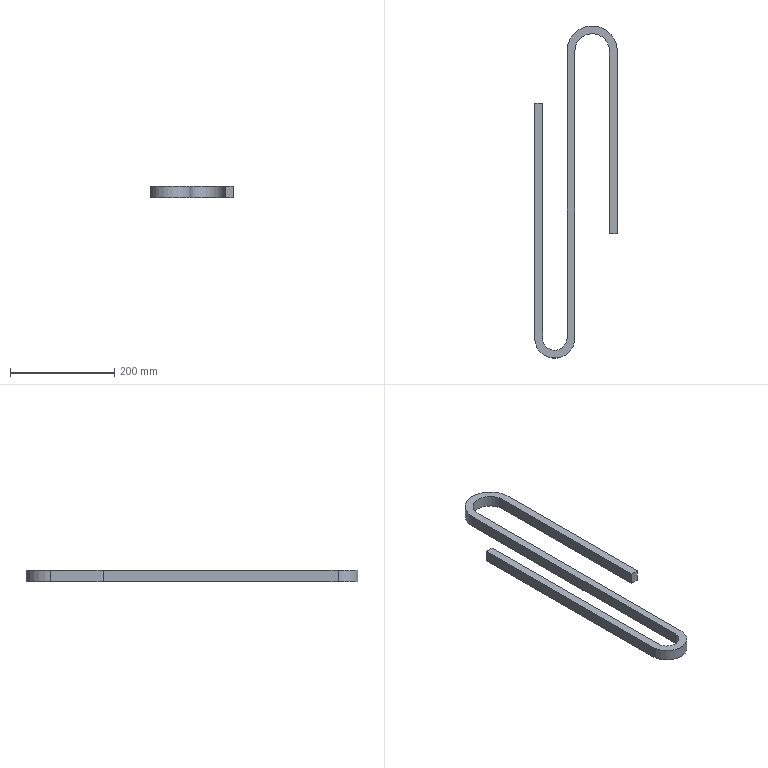Part | STEP file | PN_0043 (chain bar) | 1 solid | 14 faces | box 158.46 x 636.775 x 22 mm | volume 522937 mm3 | plane 10 | cylinder 4 | commonest cylinder face diameters 46.91 x1 66.28 x1 77.09 x1 96.46 x1
STEP:
#1=CARTESIAN_POINT('',(0.,0.,0.));
#2=DIRECTION('',(0.,0.,1.));
#3=DIRECTION('',(1.,0.,0.));
#4=AXIS2_PLACEMENT_3D('',#1,#2,#3);
#5=CARTESIAN_POINT('',(-95.14,150.,11.));
#6=VERTEX_POINT('',#5);
#7=CARTESIAN_POINT('',(-95.14,150.,-11.));
#8=VERTEX_POINT('',#7);
#9=CARTESIAN_POINT('',(-95.14,150.,-11.));
#10=DIRECTION('',(0.,0.,-1.));
#11=VECTOR('',#10,1.);
#12=LINE('',#9,#11);
#13=CARTESIAN_POINT('',(-95.14,150.,-11.));
#14=DIRECTION('',(1.,0.,0.));
#15=DIRECTION('',(0.,1.,0.));
#16=AXIS2_PLACEMENT_3D('',#13,#14,#15);
#17=PLANE('',#16);
#18=CARTESIAN_POINT('',(0.,0.));
#19=DIRECTION('',(0.,-1.));
#20=VECTOR('',#19,1.);
#21=LINE('',#18,#20);
#22=(GEOMETRIC_REPRESENTATION_CONTEXT(2)PARAMETRIC_REPRESENTATION_CONTEXT()REPRESENTATION_CONTEXT('',''));
#23=DEFINITIONAL_REPRESENTATION('',(#21),#22);
#24=PCURVE('',#17,#23);
#25=CARTESIAN_POINT('',(-71.685,150.,0.));
#26=DIRECTION('',(0.,0.,-1.));
#27=DIRECTION('',(-1.,0.,0.));
#28=AXIS2_PLACEMENT_3D('',#25,#26,#27);
#29=CYLINDRICAL_SURFACE('',#28,23.455);
#30=CARTESIAN_POINT('',(6.283,11.));
#31=DIRECTION('',(0.,1.));
#32=VECTOR('',#31,1.);
#33=LINE('',#30,#32);
#34=(GEOMETRIC_REPRESENTATION_CONTEXT(2)PARAMETRIC_REPRESENTATION_CONTEXT()REPRESENTATION_CONTEXT('',''));
#35=DEFINITIONAL_REPRESENTATION('',(#33),#34);
#36=PCURVE('',#29,#35);
#37=SURFACE_CURVE('',#12,(#24,#36),.PCURVE_S1.);
#38=EDGE_CURVE('',#6,#8,#37,.T.);
#39=ORIENTED_EDGE('',*,*,#38,.T.);
#40=CARTESIAN_POINT('',(-95.14,600.,-11.));
#41=VERTEX_POINT('',#40);
#42=CARTESIAN_POINT('',(-95.14,150.,-11.));
#43=DIRECTION('',(0.,1.,0.));
#44=VECTOR('',#43,1.);
#45=LINE('',#42,#44);
#46=CARTESIAN_POINT('',(0.,0.));
#47=DIRECTION('',(1.,0.));
#48=VECTOR('',#47,1.);
#49=LINE('',#46,#48);
#50=(GEOMETRIC_REPRESENTATION_CONTEXT(2)PARAMETRIC_REPRESENTATION_CONTEXT()REPRESENTATION_CONTEXT('',''));
#51=DEFINITIONAL_REPRESENTATION('',(#49),#50);
#52=PCURVE('',#17,#51);
#53=CARTESIAN_POINT('',(48.23,700.,-11.));
#54=DIRECTION('',(0.,0.,1.));
#55=DIRECTION('',(1.,0.,0.));
#56=AXIS2_PLACEMENT_3D('',#53,#54,#55);
#57=PLANE('',#56);
#58=CARTESIAN_POINT('',(-143.37,-550.));
#59=DIRECTION('',(0.,1.));
#60=VECTOR('',#59,1.);
#61=LINE('',#58,#60);
#62=(GEOMETRIC_REPRESENTATION_CONTEXT(2)PARAMETRIC_REPRESENTATION_CONTEXT()REPRESENTATION_CONTEXT('',''));
#63=DEFINITIONAL_REPRESENTATION('',(#61),#62);
#64=PCURVE('',#57,#63);
#65=SURFACE_CURVE('',#45,(#52,#64),.PCURVE_S1.);
#66=EDGE_CURVE('',#8,#41,#65,.T.);
#67=ORIENTED_EDGE('',*,*,#66,.T.);
#68=CARTESIAN_POINT('',(-95.14,600.,11.));
#69=VERTEX_POINT('',#68);
#70=CARTESIAN_POINT('',(-95.14,600.,-11.));
#71=DIRECTION('',(0.,0.,-1.));
#72=VECTOR('',#71,1.);
#73=LINE('',#70,#72);
#74=CARTESIAN_POINT('',(450.,0.));
#75=DIRECTION('',(0.,-1.));
#76=VECTOR('',#75,1.);
#77=LINE('',#74,#76);
#78=(GEOMETRIC_REPRESENTATION_CONTEXT(2)PARAMETRIC_REPRESENTATION_CONTEXT()REPRESENTATION_CONTEXT('',''));
#79=DEFINITIONAL_REPRESENTATION('',(#77),#78);
#80=PCURVE('',#17,#79);
#81=CARTESIAN_POINT('',(-143.37,600.,0.));
#82=DIRECTION('',(0.,-1.,0.));
#83=DIRECTION('',(0.,0.,-1.));
#84=AXIS2_PLACEMENT_3D('',#81,#82,#83);
#85=PLANE('',#84);
#86=CARTESIAN_POINT('',(11.,48.23));
#87=DIRECTION('',(1.,0.));
#88=VECTOR('',#87,1.);
#89=LINE('',#86,#88);
#90=(GEOMETRIC_REPRESENTATION_CONTEXT(2)PARAMETRIC_REPRESENTATION_CONTEXT()REPRESENTATION_CONTEXT('',''));
#91=DEFINITIONAL_REPRESENTATION('',(#89),#90);
#92=PCURVE('',#85,#91);
#93=SURFACE_CURVE('',#73,(#80,#92),.PCURVE_S1.);
#94=EDGE_CURVE('',#69,#41,#93,.T.);
#95=ORIENTED_EDGE('',*,*,#94,.F.);
#96=CARTESIAN_POINT('',(-95.14,150.,11.));
#97=DIRECTION('',(0.,1.,0.));
#98=VECTOR('',#97,1.);
#99=LINE('',#96,#98);
#100=CARTESIAN_POINT('',(0.,22.));
#101=DIRECTION('',(1.,0.));
#102=VECTOR('',#101,1.);
#103=LINE('',#100,#102);
#104=(GEOMETRIC_REPRESENTATION_CONTEXT(2)PARAMETRIC_REPRESENTATION_CONTEXT()REPRESENTATION_CONTEXT('',''));
#105=DEFINITIONAL_REPRESENTATION('',(#103),#104);
#106=PCURVE('',#17,#105);
#107=CARTESIAN_POINT('',(48.23,700.,11.));
#108=DIRECTION('',(0.,0.,-1.));
#109=DIRECTION('',(-1.,0.,0.));
#110=AXIS2_PLACEMENT_3D('',#107,#108,#109);
#111=PLANE('',#110);
#112=CARTESIAN_POINT('',(143.37,-550.));
#113=DIRECTION('',(0.,1.));
#114=VECTOR('',#113,1.);
#115=LINE('',#112,#114);
#116=(GEOMETRIC_REPRESENTATION_CONTEXT(2)PARAMETRIC_REPRESENTATION_CONTEXT()REPRESENTATION_CONTEXT('',''));
#117=DEFINITIONAL_REPRESENTATION('',(#115),#116);
#118=PCURVE('',#111,#117);
#119=SURFACE_CURVE('',#99,(#106,#118),.PCURVE_S1.);
#120=EDGE_CURVE('',#6,#69,#119,.T.);
#121=ORIENTED_EDGE('',*,*,#120,.F.);
#122=EDGE_LOOP('',(#39,#67,#95,#121));
#123=FACE_BOUND('',#122,.T.);
#124=ADVANCED_FACE('',(#123),#17,.T.);
#125=CARTESIAN_POINT('',(-110.23,150.,-11.));
#126=VERTEX_POINT('',#125);
#127=CARTESIAN_POINT('',(-110.23,150.,11.));
#128=VERTEX_POINT('',#127);
#129=CARTESIAN_POINT('',(-110.23,150.,-11.));
#130=DIRECTION('',(0.,0.,1.));
#131=VECTOR('',#130,1.);
#132=LINE('',#129,#131);
#133=CARTESIAN_POINT('',(-110.23,150.,-11.));
#134=DIRECTION('',(-1.,0.,0.));
#135=DIRECTION('',(0.,-1.,0.));
#136=AXIS2_PLACEMENT_3D('',#133,#134,#135);
#137=PLANE('',#136);
#138=CARTESIAN_POINT('',(0.,0.));
#139=DIRECTION('',(0.,1.));
#140=VECTOR('',#139,1.);
#141=LINE('',#138,#140);
#142=(GEOMETRIC_REPRESENTATION_CONTEXT(2)PARAMETRIC_REPRESENTATION_CONTEXT()REPRESENTATION_CONTEXT('',''));
#143=DEFINITIONAL_REPRESENTATION('',(#141),#142);
#144=PCURVE('',#137,#143);
#145=CARTESIAN_POINT('',(-71.685,150.,0.));
#146=DIRECTION('',(0.,0.,-1.));
#147=DIRECTION('',(-1.,0.,0.));
#148=AXIS2_PLACEMENT_3D('',#145,#146,#147);
#149=CYLINDRICAL_SURFACE('',#148,38.545);
#150=CARTESIAN_POINT('',(6.283,11.));
#151=DIRECTION('',(0.,-1.));
#152=VECTOR('',#151,1.);
#153=LINE('',#150,#152);
#154=(GEOMETRIC_REPRESENTATION_CONTEXT(2)PARAMETRIC_REPRESENTATION_CONTEXT()REPRESENTATION_CONTEXT('',''));
#155=DEFINITIONAL_REPRESENTATION('',(#153),#154);
#156=PCURVE('',#149,#155);
#157=SURFACE_CURVE('',#132,(#144,#156),.PCURVE_S1.);
#158=EDGE_CURVE('',#126,#128,#157,.T.);
#159=ORIENTED_EDGE('',*,*,#158,.T.);
#160=CARTESIAN_POINT('',(-110.23,600.,11.));
#161=VERTEX_POINT('',#160);
#162=CARTESIAN_POINT('',(-110.23,150.,11.));
#163=DIRECTION('',(0.,1.,0.));
#164=VECTOR('',#163,1.);
#165=LINE('',#162,#164);
#166=CARTESIAN_POINT('',(0.,22.));
#167=DIRECTION('',(-1.,0.));
#168=VECTOR('',#167,1.);
#169=LINE('',#166,#168);
#170=(GEOMETRIC_REPRESENTATION_CONTEXT(2)PARAMETRIC_REPRESENTATION_CONTEXT()REPRESENTATION_CONTEXT('',''));
#171=DEFINITIONAL_REPRESENTATION('',(#169),#170);
#172=PCURVE('',#137,#171);
#173=CARTESIAN_POINT('',(158.46,-550.));
#174=DIRECTION('',(0.,1.));
#175=VECTOR('',#174,1.);
#176=LINE('',#173,#175);
#177=(GEOMETRIC_REPRESENTATION_CONTEXT(2)PARAMETRIC_REPRESENTATION_CONTEXT()REPRESENTATION_CONTEXT('',''));
#178=DEFINITIONAL_REPRESENTATION('',(#176),#177);
#179=PCURVE('',#111,#178);
#180=SURFACE_CURVE('',#165,(#172,#179),.PCURVE_S1.);
#181=EDGE_CURVE('',#128,#161,#180,.T.);
#182=ORIENTED_EDGE('',*,*,#181,.T.);
#183=CARTESIAN_POINT('',(-110.23,600.,-11.));
#184=VERTEX_POINT('',#183);
#185=CARTESIAN_POINT('',(-110.23,600.,-11.));
#186=DIRECTION('',(0.,0.,1.));
#187=VECTOR('',#186,1.);
#188=LINE('',#185,#187);
#189=CARTESIAN_POINT('',(-450.,0.));
#190=DIRECTION('',(0.,1.));
#191=VECTOR('',#190,1.);
#192=LINE('',#189,#191);
#193=(GEOMETRIC_REPRESENTATION_CONTEXT(2)PARAMETRIC_REPRESENTATION_CONTEXT()REPRESENTATION_CONTEXT('',''));
#194=DEFINITIONAL_REPRESENTATION('',(#192),#193);
#195=PCURVE('',#137,#194);
#196=CARTESIAN_POINT('',(11.,33.14));
#197=DIRECTION('',(-1.,0.));
#198=VECTOR('',#197,1.);
#199=LINE('',#196,#198);
#200=(GEOMETRIC_REPRESENTATION_CONTEXT(2)PARAMETRIC_REPRESENTATION_CONTEXT()REPRESENTATION_CONTEXT('',''));
#201=DEFINITIONAL_REPRESENTATION('',(#199),#200);
#202=PCURVE('',#85,#201);
#203=SURFACE_CURVE('',#188,(#195,#202),.PCURVE_S1.);
#204=EDGE_CURVE('',#184,#161,#203,.T.);
#205=ORIENTED_EDGE('',*,*,#204,.F.);
#206=CARTESIAN_POINT('',(-110.23,150.,-11.));
#207=DIRECTION('',(0.,1.,0.));
#208=VECTOR('',#207,1.);
#209=LINE('',#206,#208);
#210=CARTESIAN_POINT('',(0.,0.));
#211=DIRECTION('',(-1.,0.));
#212=VECTOR('',#211,1.);
#213=LINE('',#210,#212);
#214=(GEOMETRIC_REPRESENTATION_CONTEXT(2)PARAMETRIC_REPRESENTATION_CONTEXT()REPRESENTATION_CONTEXT('',''));
#215=DEFINITIONAL_REPRESENTATION('',(#213),#214);
#216=PCURVE('',#137,#215);
#217=CARTESIAN_POINT('',(-158.46,-550.));
#218=DIRECTION('',(0.,1.));
#219=VECTOR('',#218,1.);
#220=LINE('',#217,#219);
#221=(GEOMETRIC_REPRESENTATION_CONTEXT(2)PARAMETRIC_REPRESENTATION_CONTEXT()REPRESENTATION_CONTEXT('',''));
#222=DEFINITIONAL_REPRESENTATION('',(#220),#221);
#223=PCURVE('',#57,#222);
#224=SURFACE_CURVE('',#209,(#216,#223),.PCURVE_S1.);
#225=EDGE_CURVE('',#126,#184,#224,.T.);
#226=ORIENTED_EDGE('',*,*,#225,.F.);
#227=EDGE_LOOP('',(#159,#182,#205,#226));
#228=FACE_BOUND('',#227,.T.);
#229=ADVANCED_FACE('',(#228),#137,.T.);
#230=CARTESIAN_POINT('',(-48.23,150.,11.));
#231=VERTEX_POINT('',#230);
#232=CARTESIAN_POINT('',(-71.685,150.,11.));
#233=DIRECTION('',(0.,0.,-1.));
#234=DIRECTION('',(-1.,0.,0.));
#235=AXIS2_PLACEMENT_3D('',#232,#233,#234);
#236=CIRCLE('',#235,23.455);
#237=CARTESIAN_POINT('',(0.,-11.));
#238=DIRECTION('',(1.,0.));
#239=VECTOR('',#238,1.);
#240=LINE('',#237,#239);
#241=(GEOMETRIC_REPRESENTATION_CONTEXT(2)PARAMETRIC_REPRESENTATION_CONTEXT()REPRESENTATION_CONTEXT('',''));
#242=DEFINITIONAL_REPRESENTATION('',(#240),#241);
#243=PCURVE('',#29,#242);
#244=CARTESIAN_POINT('',(119.915,-550.));
#245=DIRECTION('',(1.,0.));
#246=AXIS2_PLACEMENT_2D('',#244,#245);
#247=CIRCLE('',#246,23.455);
#248=(GEOMETRIC_REPRESENTATION_CONTEXT(2)PARAMETRIC_REPRESENTATION_CONTEXT()REPRESENTATION_CONTEXT('',''));
#249=DEFINITIONAL_REPRESENTATION('',(#247),#248);
#250=PCURVE('',#111,#249);
#251=SURFACE_CURVE('',#236,(#243,#250),.PCURVE_S1.);
#252=EDGE_CURVE('',#231,#6,#251,.T.);
#253=ORIENTED_EDGE('',*,*,#252,.T.);
#254=ORIENTED_EDGE('',*,*,#38,.T.);
#255=CARTESIAN_POINT('',(-48.23,150.,-11.));
#256=VERTEX_POINT('',#255);
#257=CARTESIAN_POINT('',(-71.685,150.,-11.));
#258=DIRECTION('',(0.,0.,-1.));
#259=DIRECTION('',(-1.,0.,0.));
#260=AXIS2_PLACEMENT_3D('',#257,#258,#259);
#261=CIRCLE('',#260,23.455);
#262=CARTESIAN_POINT('',(0.,11.));
#263=DIRECTION('',(1.,0.));
#264=VECTOR('',#263,1.);
#265=LINE('',#262,#264);
#266=(GEOMETRIC_REPRESENTATION_CONTEXT(2)PARAMETRIC_REPRESENTATION_CONTEXT()REPRESENTATION_CONTEXT('',''));
#267=DEFINITIONAL_REPRESENTATION('',(#265),#266);
#268=PCURVE('',#29,#267);
#269=CARTESIAN_POINT('',(-143.37,-550.));
#270=CARTESIAN_POINT('',(-143.37,-509.375));
#271=CARTESIAN_POINT('',(-108.188,-529.687));
#272=CARTESIAN_POINT('',(-73.005,-550.));
#273=CARTESIAN_POINT('',(-108.188,-570.313));
#274=CARTESIAN_POINT('',(-143.37,-590.625));
#275=CARTESIAN_POINT('',(-143.37,-550.));
#276=(BOUNDED_CURVE()B_SPLINE_CURVE(2,(#269,#270,#271,#272,#273,#274,#275),.UNSPECIFIED.,.T.,.F.)B_SPLINE_CURVE_WITH_KNOTS((1,2,2,2,2,1),(-2.094,0.,2.094,4.189,6.283,8.378),.UNSPECIFIED.)CURVE()GEOMETRIC_REPRESENTATION_ITEM()RATIONAL_B_SPLINE_CURVE((1.,0.5,1.,0.5,1.,0.5,1.))REPRESENTATION_ITEM(''));
#277=(GEOMETRIC_REPRESENTATION_CONTEXT(2)PARAMETRIC_REPRESENTATION_CONTEXT()REPRESENTATION_CONTEXT('',''));
#278=DEFINITIONAL_REPRESENTATION('',(#276),#277);
#279=PCURVE('',#57,#278);
#280=SURFACE_CURVE('',#261,(#268,#279),.PCURVE_S1.);
#281=EDGE_CURVE('',#256,#8,#280,.T.);
#282=ORIENTED_EDGE('',*,*,#281,.F.);
#283=CARTESIAN_POINT('',(-48.23,150.,-11.));
#284=DIRECTION('',(0.,0.,-1.));
#285=VECTOR('',#284,1.);
#286=LINE('',#283,#285);
#287=CARTESIAN_POINT('',(3.142,11.));
#288=DIRECTION('',(0.,1.));
#289=VECTOR('',#288,1.);
#290=LINE('',#287,#289);
#291=(GEOMETRIC_REPRESENTATION_CONTEXT(2)PARAMETRIC_REPRESENTATION_CONTEXT()REPRESENTATION_CONTEXT('',''));
#292=DEFINITIONAL_REPRESENTATION('',(#290),#291);
#293=PCURVE('',#29,#292);
#294=CARTESIAN_POINT('',(-48.23,700.,-11.));
#295=DIRECTION('',(-1.,0.,0.));
#296=DIRECTION('',(0.,-1.,0.));
#297=AXIS2_PLACEMENT_3D('',#294,#295,#296);
#298=PLANE('',#297);
#299=CARTESIAN_POINT('',(550.,0.));
#300=DIRECTION('',(0.,-1.));
#301=VECTOR('',#300,1.);
#302=LINE('',#299,#301);
#303=(GEOMETRIC_REPRESENTATION_CONTEXT(2)PARAMETRIC_REPRESENTATION_CONTEXT()REPRESENTATION_CONTEXT('',''));
#304=DEFINITIONAL_REPRESENTATION('',(#302),#303);
#305=PCURVE('',#298,#304);
#306=SURFACE_CURVE('',#286,(#293,#305),.PCURVE_S1.);
#307=EDGE_CURVE('',#231,#256,#306,.T.);
#308=ORIENTED_EDGE('',*,*,#307,.F.);
#309=EDGE_LOOP('',(#253,#254,#282,#308));
#310=FACE_BOUND('',#309,.F.);
#311=ADVANCED_FACE('',(#310),#29,.F.);
#312=CARTESIAN_POINT('',(-33.14,150.,-11.));
#313=VERTEX_POINT('',#312);
#314=CARTESIAN_POINT('',(-33.14,150.,11.));
#315=VERTEX_POINT('',#314);
#316=CARTESIAN_POINT('',(-33.14,150.,-11.));
#317=DIRECTION('',(0.,0.,1.));
#318=VECTOR('',#317,1.);
#319=LINE('',#316,#318);
#320=CARTESIAN_POINT('',(3.142,11.));
#321=DIRECTION('',(0.,-1.));
#322=VECTOR('',#321,1.);
#323=LINE('',#320,#322);
#324=(GEOMETRIC_REPRESENTATION_CONTEXT(2)PARAMETRIC_REPRESENTATION_CONTEXT()REPRESENTATION_CONTEXT('',''));
#325=DEFINITIONAL_REPRESENTATION('',(#323),#324);
#326=PCURVE('',#149,#325);
#327=CARTESIAN_POINT('',(-33.14,700.,-11.));
#328=DIRECTION('',(1.,0.,0.));
#329=DIRECTION('',(0.,1.,0.));
#330=AXIS2_PLACEMENT_3D('',#327,#328,#329);
#331=PLANE('',#330);
#332=CARTESIAN_POINT('',(-550.,0.));
#333=DIRECTION('',(0.,1.));
#334=VECTOR('',#333,1.);
#335=LINE('',#332,#334);
#336=(GEOMETRIC_REPRESENTATION_CONTEXT(2)PARAMETRIC_REPRESENTATION_CONTEXT()REPRESENTATION_CONTEXT('',''));
#337=DEFINITIONAL_REPRESENTATION('',(#335),#336);
#338=PCURVE('',#331,#337);
#339=SURFACE_CURVE('',#319,(#326,#338),.PCURVE_S1.);
#340=EDGE_CURVE('',#313,#315,#339,.T.);
#341=ORIENTED_EDGE('',*,*,#340,.T.);
#342=CARTESIAN_POINT('',(-71.685,150.,11.));
#343=DIRECTION('',(0.,0.,-1.));
#344=DIRECTION('',(-1.,0.,0.));
#345=AXIS2_PLACEMENT_3D('',#342,#343,#344);
#346=CIRCLE('',#345,38.545);
#347=CARTESIAN_POINT('',(0.,-11.));
#348=DIRECTION('',(1.,0.));
#349=VECTOR('',#348,1.);
#350=LINE('',#347,#349);
#351=(GEOMETRIC_REPRESENTATION_CONTEXT(2)PARAMETRIC_REPRESENTATION_CONTEXT()REPRESENTATION_CONTEXT('',''));
#352=DEFINITIONAL_REPRESENTATION('',(#350),#351);
#353=PCURVE('',#149,#352);
#354=CARTESIAN_POINT('',(119.915,-550.));
#355=DIRECTION('',(1.,0.));
#356=AXIS2_PLACEMENT_2D('',#354,#355);
#357=CIRCLE('',#356,38.545);
#358=(GEOMETRIC_REPRESENTATION_CONTEXT(2)PARAMETRIC_REPRESENTATION_CONTEXT()REPRESENTATION_CONTEXT('',''));
#359=DEFINITIONAL_REPRESENTATION('',(#357),#358);
#360=PCURVE('',#111,#359);
#361=SURFACE_CURVE('',#346,(#353,#360),.PCURVE_S1.);
#362=EDGE_CURVE('',#315,#128,#361,.T.);
#363=ORIENTED_EDGE('',*,*,#362,.T.);
#364=ORIENTED_EDGE('',*,*,#158,.F.);
#365=CARTESIAN_POINT('',(-71.685,150.,-11.));
#366=DIRECTION('',(0.,0.,-1.));
#367=DIRECTION('',(-1.,0.,0.));
#368=AXIS2_PLACEMENT_3D('',#365,#366,#367);
#369=CIRCLE('',#368,38.545);
#370=CARTESIAN_POINT('',(0.,11.));
#371=DIRECTION('',(1.,0.));
#372=VECTOR('',#371,1.);
#373=LINE('',#370,#372);
#374=(GEOMETRIC_REPRESENTATION_CONTEXT(2)PARAMETRIC_REPRESENTATION_CONTEXT()REPRESENTATION_CONTEXT('',''));
#375=DEFINITIONAL_REPRESENTATION('',(#373),#374);
#376=PCURVE('',#149,#375);
#377=CARTESIAN_POINT('',(-158.46,-550.));
#378=CARTESIAN_POINT('',(-158.46,-483.238));
#379=CARTESIAN_POINT('',(-100.642,-516.619));
#380=CARTESIAN_POINT('',(-42.825,-550.));
#381=CARTESIAN_POINT('',(-100.642,-583.381));
#382=CARTESIAN_POINT('',(-158.46,-616.762));
#383=CARTESIAN_POINT('',(-158.46,-550.));
#384=(BOUNDED_CURVE()B_SPLINE_CURVE(2,(#377,#378,#379,#380,#381,#382,#383),.UNSPECIFIED.,.T.,.F.)B_SPLINE_CURVE_WITH_KNOTS((1,2,2,2,2,1),(-2.094,0.,2.094,4.189,6.283,8.378),.UNSPECIFIED.)CURVE()GEOMETRIC_REPRESENTATION_ITEM()RATIONAL_B_SPLINE_CURVE((1.,0.5,1.,0.5,1.,0.5,1.))REPRESENTATION_ITEM(''));
#385=(GEOMETRIC_REPRESENTATION_CONTEXT(2)PARAMETRIC_REPRESENTATION_CONTEXT()REPRESENTATION_CONTEXT('',''));
#386=DEFINITIONAL_REPRESENTATION('',(#384),#385);
#387=PCURVE('',#57,#386);
#388=SURFACE_CURVE('',#369,(#376,#387),.PCURVE_S1.);
#389=EDGE_CURVE('',#313,#126,#388,.T.);
#390=ORIENTED_EDGE('',*,*,#389,.F.);
#391=EDGE_LOOP('',(#341,#363,#364,#390));
#392=FACE_BOUND('',#391,.T.);
#393=ADVANCED_FACE('',(#392),#149,.T.);
#394=CARTESIAN_POINT('',(-48.23,700.,11.));
#395=VERTEX_POINT('',#394);
#396=CARTESIAN_POINT('',(-48.23,700.,-11.));
#397=VERTEX_POINT('',#396);
#398=CARTESIAN_POINT('',(-48.23,700.,-11.));
#399=DIRECTION('',(0.,0.,-1.));
#400=VECTOR('',#399,1.);
#401=LINE('',#398,#400);
#402=CARTESIAN_POINT('',(0.,0.));
#403=DIRECTION('',(0.,-1.));
#404=VECTOR('',#403,1.);
#405=LINE('',#402,#404);
#406=(GEOMETRIC_REPRESENTATION_CONTEXT(2)PARAMETRIC_REPRESENTATION_CONTEXT()REPRESENTATION_CONTEXT('',''));
#407=DEFINITIONAL_REPRESENTATION('',(#405),#406);
#408=PCURVE('',#298,#407);
#409=CARTESIAN_POINT('',(0.,700.,0.));
#410=DIRECTION('',(0.,0.,1.));
#411=DIRECTION('',(1.,0.,0.));
#412=AXIS2_PLACEMENT_3D('',#409,#410,#411);
#413=CYLINDRICAL_SURFACE('',#412,48.23);
#414=CARTESIAN_POINT('',(3.142,-11.));
#415=DIRECTION('',(0.,-1.));
#416=VECTOR('',#415,1.);
#417=LINE('',#414,#416);
#418=(GEOMETRIC_REPRESENTATION_CONTEXT(2)PARAMETRIC_REPRESENTATION_CONTEXT()REPRESENTATION_CONTEXT('',''));
#419=DEFINITIONAL_REPRESENTATION('',(#417),#418);
#420=PCURVE('',#413,#419);
#421=SURFACE_CURVE('',#401,(#408,#420),.PCURVE_S1.);
#422=EDGE_CURVE('',#395,#397,#421,.T.);
#423=ORIENTED_EDGE('',*,*,#422,.T.);
#424=CARTESIAN_POINT('',(-48.23,700.,-11.));
#425=DIRECTION('',(0.,-1.,0.));
#426=VECTOR('',#425,1.);
#427=LINE('',#424,#426);
#428=CARTESIAN_POINT('',(0.,0.));
#429=DIRECTION('',(1.,0.));
#430=VECTOR('',#429,1.);
#431=LINE('',#428,#430);
#432=(GEOMETRIC_REPRESENTATION_CONTEXT(2)PARAMETRIC_REPRESENTATION_CONTEXT()REPRESENTATION_CONTEXT('',''));
#433=DEFINITIONAL_REPRESENTATION('',(#431),#432);
#434=PCURVE('',#298,#433);
#435=CARTESIAN_POINT('',(-96.46,0.));
#436=DIRECTION('',(0.,-1.));
#437=VECTOR('',#436,1.);
#438=LINE('',#435,#437);
#439=(GEOMETRIC_REPRESENTATION_CONTEXT(2)PARAMETRIC_REPRESENTATION_CONTEXT()REPRESENTATION_CONTEXT('',''));
#440=DEFINITIONAL_REPRESENTATION('',(#438),#439);
#441=PCURVE('',#57,#440);
#442=SURFACE_CURVE('',#427,(#434,#441),.PCURVE_S1.);
#443=EDGE_CURVE('',#397,#256,#442,.T.);
#444=ORIENTED_EDGE('',*,*,#443,.T.);
#445=ORIENTED_EDGE('',*,*,#307,.F.);
#446=CARTESIAN_POINT('',(-48.23,700.,11.));
#447=DIRECTION('',(0.,-1.,0.));
#448=VECTOR('',#447,1.);
#449=LINE('',#446,#448);
#450=CARTESIAN_POINT('',(0.,22.));
#451=DIRECTION('',(1.,0.));
#452=VECTOR('',#451,1.);
#453=LINE('',#450,#452);
#454=(GEOMETRIC_REPRESENTATION_CONTEXT(2)PARAMETRIC_REPRESENTATION_CONTEXT()REPRESENTATION_CONTEXT('',''));
#455=DEFINITIONAL_REPRESENTATION('',(#453),#454);
#456=PCURVE('',#298,#455);
#457=CARTESIAN_POINT('',(96.46,0.));
#458=DIRECTION('',(0.,-1.));
#459=VECTOR('',#458,1.);
#460=LINE('',#457,#459);
#461=(GEOMETRIC_REPRESENTATION_CONTEXT(2)PARAMETRIC_REPRESENTATION_CONTEXT()REPRESENTATION_CONTEXT('',''));
#462=DEFINITIONAL_REPRESENTATION('',(#460),#461);
#463=PCURVE('',#111,#462);
#464=SURFACE_CURVE('',#449,(#456,#463),.PCURVE_S1.);
#465=EDGE_CURVE('',#395,#231,#464,.T.);
#466=ORIENTED_EDGE('',*,*,#465,.F.);
#467=EDGE_LOOP('',(#423,#444,#445,#466));
#468=FACE_BOUND('',#467,.T.);
#469=ADVANCED_FACE('',(#468),#298,.T.);
#470=CARTESIAN_POINT('',(-33.14,700.,-11.));
#471=VERTEX_POINT('',#470);
#472=CARTESIAN_POINT('',(-33.14,700.,11.));
#473=VERTEX_POINT('',#472);
#474=CARTESIAN_POINT('',(-33.14,700.,-11.));
#475=DIRECTION('',(0.,0.,1.));
#476=VECTOR('',#475,1.);
#477=LINE('',#474,#476);
#478=CARTESIAN_POINT('',(0.,0.));
#479=DIRECTION('',(0.,1.));
#480=VECTOR('',#479,1.);
#481=LINE('',#478,#480);
#482=(GEOMETRIC_REPRESENTATION_CONTEXT(2)PARAMETRIC_REPRESENTATION_CONTEXT()REPRESENTATION_CONTEXT('',''));
#483=DEFINITIONAL_REPRESENTATION('',(#481),#482);
#484=PCURVE('',#331,#483);
#485=CARTESIAN_POINT('',(0.,700.,0.));
#486=DIRECTION('',(0.,0.,1.));
#487=DIRECTION('',(1.,0.,0.));
#488=AXIS2_PLACEMENT_3D('',#485,#486,#487);
#489=CYLINDRICAL_SURFACE('',#488,33.14);
#490=CARTESIAN_POINT('',(3.142,-11.));
#491=DIRECTION('',(0.,1.));
#492=VECTOR('',#491,1.);
#493=LINE('',#490,#492);
#494=(GEOMETRIC_REPRESENTATION_CONTEXT(2)PARAMETRIC_REPRESENTATION_CONTEXT()REPRESENTATION_CONTEXT('',''));
#495=DEFINITIONAL_REPRESENTATION('',(#493),#494);
#496=PCURVE('',#489,#495);
#497=SURFACE_CURVE('',#477,(#484,#496),.PCURVE_S1.);
#498=EDGE_CURVE('',#471,#473,#497,.T.);
#499=ORIENTED_EDGE('',*,*,#498,.T.);
#500=CARTESIAN_POINT('',(-33.14,700.,11.));
#501=DIRECTION('',(0.,-1.,0.));
#502=VECTOR('',#501,1.);
#503=LINE('',#500,#502);
#504=CARTESIAN_POINT('',(0.,22.));
#505=DIRECTION('',(-1.,0.));
#506=VECTOR('',#505,1.);
#507=LINE('',#504,#506);
#508=(GEOMETRIC_REPRESENTATION_CONTEXT(2)PARAMETRIC_REPRESENTATION_CONTEXT()REPRESENTATION_CONTEXT('',''));
#509=DEFINITIONAL_REPRESENTATION('',(#507),#508);
#510=PCURVE('',#331,#509);
#511=CARTESIAN_POINT('',(81.37,0.));
#512=DIRECTION('',(0.,-1.));
#513=VECTOR('',#512,1.);
#514=LINE('',#511,#513);
#515=(GEOMETRIC_REPRESENTATION_CONTEXT(2)PARAMETRIC_REPRESENTATION_CONTEXT()REPRESENTATION_CONTEXT('',''));
#516=DEFINITIONAL_REPRESENTATION('',(#514),#515);
#517=PCURVE('',#111,#516);
#518=SURFACE_CURVE('',#503,(#510,#517),.PCURVE_S1.);
#519=EDGE_CURVE('',#473,#315,#518,.T.);
#520=ORIENTED_EDGE('',*,*,#519,.T.);
#521=ORIENTED_EDGE('',*,*,#340,.F.);
#522=CARTESIAN_POINT('',(-33.14,700.,-11.));
#523=DIRECTION('',(0.,-1.,0.));
#524=VECTOR('',#523,1.);
#525=LINE('',#522,#524);
#526=CARTESIAN_POINT('',(0.,0.));
#527=DIRECTION('',(-1.,0.));
#528=VECTOR('',#527,1.);
#529=LINE('',#526,#528);
#530=(GEOMETRIC_REPRESENTATION_CONTEXT(2)PARAMETRIC_REPRESENTATION_CONTEXT()REPRESENTATION_CONTEXT('',''));
#531=DEFINITIONAL_REPRESENTATION('',(#529),#530);
#532=PCURVE('',#331,#531);
#533=CARTESIAN_POINT('',(-81.37,0.));
#534=DIRECTION('',(0.,-1.));
#535=VECTOR('',#534,1.);
#536=LINE('',#533,#535);
#537=(GEOMETRIC_REPRESENTATION_CONTEXT(2)PARAMETRIC_REPRESENTATION_CONTEXT()REPRESENTATION_CONTEXT('',''));
#538=DEFINITIONAL_REPRESENTATION('',(#536),#537);
#539=PCURVE('',#57,#538);
#540=SURFACE_CURVE('',#525,(#532,#539),.PCURVE_S1.);
#541=EDGE_CURVE('',#471,#313,#540,.T.);
#542=ORIENTED_EDGE('',*,*,#541,.F.);
#543=EDGE_LOOP('',(#499,#520,#521,#542));
#544=FACE_BOUND('',#543,.T.);
#545=ADVANCED_FACE('',(#544),#331,.T.);
#546=CARTESIAN_POINT('',(48.23,700.,11.));
#547=VERTEX_POINT('',#546);
#548=CARTESIAN_POINT('',(48.23,700.,-11.));
#549=VERTEX_POINT('',#548);
#550=CARTESIAN_POINT('',(48.23,700.,-11.));
#551=DIRECTION('',(0.,0.,-1.));
#552=VECTOR('',#551,1.);
#553=LINE('',#550,#552);
#554=CARTESIAN_POINT('',(0.,-11.));
#555=DIRECTION('',(0.,-1.));
#556=VECTOR('',#555,1.);
#557=LINE('',#554,#556);
#558=(GEOMETRIC_REPRESENTATION_CONTEXT(2)PARAMETRIC_REPRESENTATION_CONTEXT()REPRESENTATION_CONTEXT('',''));
#559=DEFINITIONAL_REPRESENTATION('',(#557),#558);
#560=PCURVE('',#413,#559);
#561=CARTESIAN_POINT('',(48.23,700.,-11.));
#562=DIRECTION('',(-1.,0.,0.));
#563=DIRECTION('',(0.,-1.,0.));
#564=AXIS2_PLACEMENT_3D('',#561,#562,#563);
#565=PLANE('',#564);
#566=CARTESIAN_POINT('',(0.,0.));
#567=DIRECTION('',(0.,-1.));
#568=VECTOR('',#567,1.);
#569=LINE('',#566,#568);
#570=(GEOMETRIC_REPRESENTATION_CONTEXT(2)PARAMETRIC_REPRESENTATION_CONTEXT()REPRESENTATION_CONTEXT('',''));
#571=DEFINITIONAL_REPRESENTATION('',(#569),#570);
#572=PCURVE('',#565,#571);
#573=SURFACE_CURVE('',#553,(#560,#572),.PCURVE_S1.);
#574=EDGE_CURVE('',#547,#549,#573,.T.);
#575=ORIENTED_EDGE('',*,*,#574,.T.);
#576=CARTESIAN_POINT('',(0.,700.,-11.));
#577=DIRECTION('',(0.,0.,1.));
#578=DIRECTION('',(1.,0.,0.));
#579=AXIS2_PLACEMENT_3D('',#576,#577,#578);
#580=CIRCLE('',#579,48.23);
#581=CARTESIAN_POINT('',(0.,-11.));
#582=DIRECTION('',(1.,0.));
#583=VECTOR('',#582,1.);
#584=LINE('',#581,#583);
#585=(GEOMETRIC_REPRESENTATION_CONTEXT(2)PARAMETRIC_REPRESENTATION_CONTEXT()REPRESENTATION_CONTEXT('',''));
#586=DEFINITIONAL_REPRESENTATION('',(#584),#585);
#587=PCURVE('',#413,#586);
#588=CARTESIAN_POINT('',(-48.23,0.));
#589=DIRECTION('',(1.,0.));
#590=AXIS2_PLACEMENT_2D('',#588,#589);
#591=CIRCLE('',#590,48.23);
#592=(GEOMETRIC_REPRESENTATION_CONTEXT(2)PARAMETRIC_REPRESENTATION_CONTEXT()REPRESENTATION_CONTEXT('',''));
#593=DEFINITIONAL_REPRESENTATION('',(#591),#592);
#594=PCURVE('',#57,#593);
#595=SURFACE_CURVE('',#580,(#587,#594),.PCURVE_S1.);
#596=EDGE_CURVE('',#549,#397,#595,.T.);
#597=ORIENTED_EDGE('',*,*,#596,.T.);
#598=ORIENTED_EDGE('',*,*,#422,.F.);
#599=CARTESIAN_POINT('',(0.,700.,11.));
#600=DIRECTION('',(0.,0.,1.));
#601=DIRECTION('',(1.,0.,0.));
#602=AXIS2_PLACEMENT_3D('',#599,#600,#601);
#603=CIRCLE('',#602,48.23);
#604=CARTESIAN_POINT('',(0.,11.));
#605=DIRECTION('',(1.,0.));
#606=VECTOR('',#605,1.);
#607=LINE('',#604,#606);
#608=(GEOMETRIC_REPRESENTATION_CONTEXT(2)PARAMETRIC_REPRESENTATION_CONTEXT()REPRESENTATION_CONTEXT('',''));
#609=DEFINITIONAL_REPRESENTATION('',(#607),#608);
#610=PCURVE('',#413,#609);
#611=CARTESIAN_POINT('',(0.,0.));
#612=CARTESIAN_POINT('',(0.,83.537));
#613=CARTESIAN_POINT('',(72.345,41.768));
#614=CARTESIAN_POINT('',(144.69,0.));
#615=CARTESIAN_POINT('',(72.345,-41.768));
#616=CARTESIAN_POINT('',(0.,-83.537));
#617=CARTESIAN_POINT('',(0.,0.));
#618=(BOUNDED_CURVE()B_SPLINE_CURVE(2,(#611,#612,#613,#614,#615,#616,#617),.UNSPECIFIED.,.T.,.F.)B_SPLINE_CURVE_WITH_KNOTS((1,2,2,2,2,1),(-2.094,0.,2.094,4.189,6.283,8.378),.UNSPECIFIED.)CURVE()GEOMETRIC_REPRESENTATION_ITEM()RATIONAL_B_SPLINE_CURVE((1.,0.5,1.,0.5,1.,0.5,1.))REPRESENTATION_ITEM(''));
#619=(GEOMETRIC_REPRESENTATION_CONTEXT(2)PARAMETRIC_REPRESENTATION_CONTEXT()REPRESENTATION_CONTEXT('',''));
#620=DEFINITIONAL_REPRESENTATION('',(#618),#619);
#621=PCURVE('',#111,#620);
#622=SURFACE_CURVE('',#603,(#610,#621),.PCURVE_S1.);
#623=EDGE_CURVE('',#547,#395,#622,.T.);
#624=ORIENTED_EDGE('',*,*,#623,.F.);
#625=EDGE_LOOP('',(#575,#597,#598,#624));
#626=FACE_BOUND('',#625,.T.);
#627=ADVANCED_FACE('',(#626),#413,.T.);
#628=CARTESIAN_POINT('',(33.14,700.,-11.));
#629=VERTEX_POINT('',#628);
#630=CARTESIAN_POINT('',(0.,700.,-11.));
#631=DIRECTION('',(0.,0.,1.));
#632=DIRECTION('',(1.,0.,0.));
#633=AXIS2_PLACEMENT_3D('',#630,#631,#632);
#634=CIRCLE('',#633,33.14);
#635=CARTESIAN_POINT('',(0.,-11.));
#636=DIRECTION('',(1.,0.));
#637=VECTOR('',#636,1.);
#638=LINE('',#635,#637);
#639=(GEOMETRIC_REPRESENTATION_CONTEXT(2)PARAMETRIC_REPRESENTATION_CONTEXT()REPRESENTATION_CONTEXT('',''));
#640=DEFINITIONAL_REPRESENTATION('',(#638),#639);
#641=PCURVE('',#489,#640);
#642=CARTESIAN_POINT('',(-48.23,0.));
#643=DIRECTION('',(1.,0.));
#644=AXIS2_PLACEMENT_2D('',#642,#643);
#645=CIRCLE('',#644,33.14);
#646=(GEOMETRIC_REPRESENTATION_CONTEXT(2)PARAMETRIC_REPRESENTATION_CONTEXT()REPRESENTATION_CONTEXT('',''));
#647=DEFINITIONAL_REPRESENTATION('',(#645),#646);
#648=PCURVE('',#57,#647);
#649=SURFACE_CURVE('',#634,(#641,#648),.PCURVE_S1.);
#650=EDGE_CURVE('',#629,#471,#649,.T.);
#651=ORIENTED_EDGE('',*,*,#650,.T.);
#652=ORIENTED_EDGE('',*,*,#498,.T.);
#653=CARTESIAN_POINT('',(33.14,700.,11.));
#654=VERTEX_POINT('',#653);
#655=CARTESIAN_POINT('',(0.,700.,11.));
#656=DIRECTION('',(0.,0.,1.));
#657=DIRECTION('',(1.,0.,0.));
#658=AXIS2_PLACEMENT_3D('',#655,#656,#657);
#659=CIRCLE('',#658,33.14);
#660=CARTESIAN_POINT('',(0.,11.));
#661=DIRECTION('',(1.,0.));
#662=VECTOR('',#661,1.);
#663=LINE('',#660,#662);
#664=(GEOMETRIC_REPRESENTATION_CONTEXT(2)PARAMETRIC_REPRESENTATION_CONTEXT()REPRESENTATION_CONTEXT('',''));
#665=DEFINITIONAL_REPRESENTATION('',(#663),#664);
#666=PCURVE('',#489,#665);
#667=CARTESIAN_POINT('',(15.09,0.));
#668=CARTESIAN_POINT('',(15.09,57.4));
#669=CARTESIAN_POINT('',(64.8,28.7));
#670=CARTESIAN_POINT('',(114.51,0.));
#671=CARTESIAN_POINT('',(64.8,-28.7));
#672=CARTESIAN_POINT('',(15.09,-57.4));
#673=CARTESIAN_POINT('',(15.09,0.));
#674=(BOUNDED_CURVE()B_SPLINE_CURVE(2,(#667,#668,#669,#670,#671,#672,#673),.UNSPECIFIED.,.T.,.F.)B_SPLINE_CURVE_WITH_KNOTS((1,2,2,2,2,1),(-2.094,0.,2.094,4.189,6.283,8.378),.UNSPECIFIED.)CURVE()GEOMETRIC_REPRESENTATION_ITEM()RATIONAL_B_SPLINE_CURVE((1.,0.5,1.,0.5,1.,0.5,1.))REPRESENTATION_ITEM(''));
#675=(GEOMETRIC_REPRESENTATION_CONTEXT(2)PARAMETRIC_REPRESENTATION_CONTEXT()REPRESENTATION_CONTEXT('',''));
#676=DEFINITIONAL_REPRESENTATION('',(#674),#675);
#677=PCURVE('',#111,#676);
#678=SURFACE_CURVE('',#659,(#666,#677),.PCURVE_S1.);
#679=EDGE_CURVE('',#654,#473,#678,.T.);
#680=ORIENTED_EDGE('',*,*,#679,.F.);
#681=CARTESIAN_POINT('',(33.14,700.,-11.));
#682=DIRECTION('',(0.,0.,1.));
#683=VECTOR('',#682,1.);
#684=LINE('',#681,#683);
#685=CARTESIAN_POINT('',(0.,-11.));
#686=DIRECTION('',(0.,1.));
#687=VECTOR('',#686,1.);
#688=LINE('',#685,#687);
#689=(GEOMETRIC_REPRESENTATION_CONTEXT(2)PARAMETRIC_REPRESENTATION_CONTEXT()REPRESENTATION_CONTEXT('',''));
#690=DEFINITIONAL_REPRESENTATION('',(#688),#689);
#691=PCURVE('',#489,#690);
#692=CARTESIAN_POINT('',(33.14,700.,-11.));
#693=DIRECTION('',(1.,0.,0.));
#694=DIRECTION('',(0.,1.,0.));
#695=AXIS2_PLACEMENT_3D('',#692,#693,#694);
#696=PLANE('',#695);
#697=CARTESIAN_POINT('',(0.,0.));
#698=DIRECTION('',(0.,1.));
#699=VECTOR('',#698,1.);
#700=LINE('',#697,#699);
#701=(GEOMETRIC_REPRESENTATION_CONTEXT(2)PARAMETRIC_REPRESENTATION_CONTEXT()REPRESENTATION_CONTEXT('',''));
#702=DEFINITIONAL_REPRESENTATION('',(#700),#701);
#703=PCURVE('',#696,#702);
#704=SURFACE_CURVE('',#684,(#691,#703),.PCURVE_S1.);
#705=EDGE_CURVE('',#629,#654,#704,.T.);
#706=ORIENTED_EDGE('',*,*,#705,.F.);
#707=EDGE_LOOP('',(#651,#652,#680,#706));
#708=FACE_BOUND('',#707,.F.);
#709=ADVANCED_FACE('',(#708),#489,.F.);
#710=CARTESIAN_POINT('',(33.14,350.,-11.));
#711=VERTEX_POINT('',#710);
#712=CARTESIAN_POINT('',(33.14,350.,11.));
#713=VERTEX_POINT('',#712);
#714=CARTESIAN_POINT('',(33.14,350.,-11.));
#715=DIRECTION('',(0.,0.,1.));
#716=VECTOR('',#715,1.);
#717=LINE('',#714,#716);
#718=CARTESIAN_POINT('',(-350.,0.));
#719=DIRECTION('',(0.,1.));
#720=VECTOR('',#719,1.);
#721=LINE('',#718,#720);
#722=(GEOMETRIC_REPRESENTATION_CONTEXT(2)PARAMETRIC_REPRESENTATION_CONTEXT()REPRESENTATION_CONTEXT('',''));
#723=DEFINITIONAL_REPRESENTATION('',(#721),#722);
#724=PCURVE('',#696,#723);
#725=CARTESIAN_POINT('',(0.,350.,0.));
#726=DIRECTION('',(0.,-1.,0.));
#727=DIRECTION('',(0.,0.,-1.));
#728=AXIS2_PLACEMENT_3D('',#725,#726,#727);
#729=PLANE('',#728);
#730=CARTESIAN_POINT('',(11.,33.14));
#731=DIRECTION('',(-1.,0.));
#732=VECTOR('',#731,1.);
#733=LINE('',#730,#732);
#734=(GEOMETRIC_REPRESENTATION_CONTEXT(2)PARAMETRIC_REPRESENTATION_CONTEXT()REPRESENTATION_CONTEXT('',''));
#735=DEFINITIONAL_REPRESENTATION('',(#733),#734);
#736=PCURVE('',#729,#735);
#737=SURFACE_CURVE('',#717,(#724,#736),.PCURVE_S1.);
#738=EDGE_CURVE('',#711,#713,#737,.T.);
#739=ORIENTED_EDGE('',*,*,#738,.T.);
#740=CARTESIAN_POINT('',(33.14,700.,11.));
#741=DIRECTION('',(0.,-1.,0.));
#742=VECTOR('',#741,1.);
#743=LINE('',#740,#742);
#744=CARTESIAN_POINT('',(0.,22.));
#745=DIRECTION('',(-1.,0.));
#746=VECTOR('',#745,1.);
#747=LINE('',#744,#746);
#748=(GEOMETRIC_REPRESENTATION_CONTEXT(2)PARAMETRIC_REPRESENTATION_CONTEXT()REPRESENTATION_CONTEXT('',''));
#749=DEFINITIONAL_REPRESENTATION('',(#747),#748);
#750=PCURVE('',#696,#749);
#751=CARTESIAN_POINT('',(15.09,0.));
#752=DIRECTION('',(0.,-1.));
#753=VECTOR('',#752,1.);
#754=LINE('',#751,#753);
#755=(GEOMETRIC_REPRESENTATION_CONTEXT(2)PARAMETRIC_REPRESENTATION_CONTEXT()REPRESENTATION_CONTEXT('',''));
#756=DEFINITIONAL_REPRESENTATION('',(#754),#755);
#757=PCURVE('',#111,#756);
#758=SURFACE_CURVE('',#743,(#750,#757),.PCURVE_S1.);
#759=EDGE_CURVE('',#654,#713,#758,.T.);
#760=ORIENTED_EDGE('',*,*,#759,.F.);
#761=ORIENTED_EDGE('',*,*,#705,.F.);
#762=CARTESIAN_POINT('',(33.14,700.,-11.));
#763=DIRECTION('',(0.,-1.,0.));
#764=VECTOR('',#763,1.);
#765=LINE('',#762,#764);
#766=CARTESIAN_POINT('',(0.,0.));
#767=DIRECTION('',(-1.,0.));
#768=VECTOR('',#767,1.);
#769=LINE('',#766,#768);
#770=(GEOMETRIC_REPRESENTATION_CONTEXT(2)PARAMETRIC_REPRESENTATION_CONTEXT()REPRESENTATION_CONTEXT('',''));
#771=DEFINITIONAL_REPRESENTATION('',(#769),#770);
#772=PCURVE('',#696,#771);
#773=CARTESIAN_POINT('',(-15.09,0.));
#774=DIRECTION('',(0.,-1.));
#775=VECTOR('',#774,1.);
#776=LINE('',#773,#775);
#777=(GEOMETRIC_REPRESENTATION_CONTEXT(2)PARAMETRIC_REPRESENTATION_CONTEXT()REPRESENTATION_CONTEXT('',''));
#778=DEFINITIONAL_REPRESENTATION('',(#776),#777);
#779=PCURVE('',#57,#778);
#780=SURFACE_CURVE('',#765,(#772,#779),.PCURVE_S1.);
#781=EDGE_CURVE('',#629,#711,#780,.T.);
#782=ORIENTED_EDGE('',*,*,#781,.T.);
#783=EDGE_LOOP('',(#739,#760,#761,#782));
#784=FACE_BOUND('',#783,.T.);
#785=ADVANCED_FACE('',(#784),#696,.F.);
#786=CARTESIAN_POINT('',(48.23,350.,11.));
#787=VERTEX_POINT('',#786);
#788=CARTESIAN_POINT('',(48.23,350.,11.));
#789=DIRECTION('',(1.,0.,0.));
#790=VECTOR('',#789,1.);
#791=LINE('',#788,#790);
#792=CARTESIAN_POINT('',(0.,-350.));
#793=DIRECTION('',(-1.,0.));
#794=VECTOR('',#793,1.);
#795=LINE('',#792,#794);
#796=(GEOMETRIC_REPRESENTATION_CONTEXT(2)PARAMETRIC_REPRESENTATION_CONTEXT()REPRESENTATION_CONTEXT('',''));
#797=DEFINITIONAL_REPRESENTATION('',(#795),#796);
#798=PCURVE('',#111,#797);
#799=CARTESIAN_POINT('',(-11.,48.23));
#800=DIRECTION('',(0.,1.));
#801=VECTOR('',#800,1.);
#802=LINE('',#799,#801);
#803=(GEOMETRIC_REPRESENTATION_CONTEXT(2)PARAMETRIC_REPRESENTATION_CONTEXT()REPRESENTATION_CONTEXT('',''));
#804=DEFINITIONAL_REPRESENTATION('',(#802),#803);
#805=PCURVE('',#729,#804);
#806=SURFACE_CURVE('',#791,(#798,#805),.PCURVE_S1.);
#807=EDGE_CURVE('',#713,#787,#806,.T.);
#808=ORIENTED_EDGE('',*,*,#807,.T.);
#809=CARTESIAN_POINT('',(48.23,700.,11.));
#810=DIRECTION('',(0.,-1.,0.));
#811=VECTOR('',#810,1.);
#812=LINE('',#809,#811);
#813=CARTESIAN_POINT('',(0.,0.));
#814=DIRECTION('',(0.,-1.));
#815=VECTOR('',#814,1.);
#816=LINE('',#813,#815);
#817=(GEOMETRIC_REPRESENTATION_CONTEXT(2)PARAMETRIC_REPRESENTATION_CONTEXT()REPRESENTATION_CONTEXT('',''));
#818=DEFINITIONAL_REPRESENTATION('',(#816),#817);
#819=PCURVE('',#111,#818);
#820=CARTESIAN_POINT('',(0.,22.));
#821=DIRECTION('',(1.,0.));
#822=VECTOR('',#821,1.);
#823=LINE('',#820,#822);
#824=(GEOMETRIC_REPRESENTATION_CONTEXT(2)PARAMETRIC_REPRESENTATION_CONTEXT()REPRESENTATION_CONTEXT('',''));
#825=DEFINITIONAL_REPRESENTATION('',(#823),#824);
#826=PCURVE('',#565,#825);
#827=SURFACE_CURVE('',#812,(#819,#826),.PCURVE_S1.);
#828=EDGE_CURVE('',#547,#787,#827,.T.);
#829=ORIENTED_EDGE('',*,*,#828,.F.);
#830=ORIENTED_EDGE('',*,*,#623,.T.);
#831=ORIENTED_EDGE('',*,*,#465,.T.);
#832=ORIENTED_EDGE('',*,*,#252,.T.);
#833=ORIENTED_EDGE('',*,*,#120,.T.);
#834=CARTESIAN_POINT('',(-95.14,600.,11.));
#835=DIRECTION('',(1.,0.,0.));
#836=VECTOR('',#835,1.);
#837=LINE('',#834,#836);
#838=CARTESIAN_POINT('',(143.37,-100.));
#839=DIRECTION('',(-1.,0.));
#840=VECTOR('',#839,1.);
#841=LINE('',#838,#840);
#842=(GEOMETRIC_REPRESENTATION_CONTEXT(2)PARAMETRIC_REPRESENTATION_CONTEXT()REPRESENTATION_CONTEXT('',''));
#843=DEFINITIONAL_REPRESENTATION('',(#841),#842);
#844=PCURVE('',#111,#843);
#845=CARTESIAN_POINT('',(-11.,48.23));
#846=DIRECTION('',(0.,1.));
#847=VECTOR('',#846,1.);
#848=LINE('',#845,#847);
#849=(GEOMETRIC_REPRESENTATION_CONTEXT(2)PARAMETRIC_REPRESENTATION_CONTEXT()REPRESENTATION_CONTEXT('',''));
#850=DEFINITIONAL_REPRESENTATION('',(#848),#849);
#851=PCURVE('',#85,#850);
#852=SURFACE_CURVE('',#837,(#844,#851),.PCURVE_S1.);
#853=EDGE_CURVE('',#161,#69,#852,.T.);
#854=ORIENTED_EDGE('',*,*,#853,.F.);
#855=ORIENTED_EDGE('',*,*,#181,.F.);
#856=ORIENTED_EDGE('',*,*,#362,.F.);
#857=ORIENTED_EDGE('',*,*,#519,.F.);
#858=ORIENTED_EDGE('',*,*,#679,.F.);
#859=ORIENTED_EDGE('',*,*,#759,.T.);
#860=EDGE_LOOP('',(#808,#829,#830,#831,#832,#833,#854,#855,#856,#857,#858,#859));
#861=FACE_BOUND('',#860,.T.);
#862=ADVANCED_FACE('',(#861),#111,.F.);
#863=CARTESIAN_POINT('',(48.23,350.,-11.));
#864=VERTEX_POINT('',#863);
#865=CARTESIAN_POINT('',(48.23,350.,-11.));
#866=DIRECTION('',(0.,0.,-1.));
#867=VECTOR('',#866,1.);
#868=LINE('',#865,#867);
#869=CARTESIAN_POINT('',(350.,0.));
#870=DIRECTION('',(0.,-1.));
#871=VECTOR('',#870,1.);
#872=LINE('',#869,#871);
#873=(GEOMETRIC_REPRESENTATION_CONTEXT(2)PARAMETRIC_REPRESENTATION_CONTEXT()REPRESENTATION_CONTEXT('',''));
#874=DEFINITIONAL_REPRESENTATION('',(#872),#873);
#875=PCURVE('',#565,#874);
#876=CARTESIAN_POINT('',(11.,48.23));
#877=DIRECTION('',(1.,0.));
#878=VECTOR('',#877,1.);
#879=LINE('',#876,#878);
#880=(GEOMETRIC_REPRESENTATION_CONTEXT(2)PARAMETRIC_REPRESENTATION_CONTEXT()REPRESENTATION_CONTEXT('',''));
#881=DEFINITIONAL_REPRESENTATION('',(#879),#880);
#882=PCURVE('',#729,#881);
#883=SURFACE_CURVE('',#868,(#875,#882),.PCURVE_S1.);
#884=EDGE_CURVE('',#787,#864,#883,.T.);
#885=ORIENTED_EDGE('',*,*,#884,.T.);
#886=CARTESIAN_POINT('',(48.23,700.,-11.));
#887=DIRECTION('',(0.,-1.,0.));
#888=VECTOR('',#887,1.);
#889=LINE('',#886,#888);
#890=CARTESIAN_POINT('',(0.,0.));
#891=DIRECTION('',(1.,0.));
#892=VECTOR('',#891,1.);
#893=LINE('',#890,#892);
#894=(GEOMETRIC_REPRESENTATION_CONTEXT(2)PARAMETRIC_REPRESENTATION_CONTEXT()REPRESENTATION_CONTEXT('',''));
#895=DEFINITIONAL_REPRESENTATION('',(#893),#894);
#896=PCURVE('',#565,#895);
#897=CARTESIAN_POINT('',(0.,0.));
#898=DIRECTION('',(0.,-1.));
#899=VECTOR('',#898,1.);
#900=LINE('',#897,#899);
#901=(GEOMETRIC_REPRESENTATION_CONTEXT(2)PARAMETRIC_REPRESENTATION_CONTEXT()REPRESENTATION_CONTEXT('',''));
#902=DEFINITIONAL_REPRESENTATION('',(#900),#901);
#903=PCURVE('',#57,#902);
#904=SURFACE_CURVE('',#889,(#896,#903),.PCURVE_S1.);
#905=EDGE_CURVE('',#549,#864,#904,.T.);
#906=ORIENTED_EDGE('',*,*,#905,.F.);
#907=ORIENTED_EDGE('',*,*,#574,.F.);
#908=ORIENTED_EDGE('',*,*,#828,.T.);
#909=EDGE_LOOP('',(#885,#906,#907,#908));
#910=FACE_BOUND('',#909,.T.);
#911=ADVANCED_FACE('',(#910),#565,.F.);
#912=CARTESIAN_POINT('',(48.23,350.,-11.));
#913=DIRECTION('',(-1.,0.,0.));
#914=VECTOR('',#913,1.);
#915=LINE('',#912,#914);
#916=CARTESIAN_POINT('',(0.,-350.));
#917=DIRECTION('',(-1.,0.));
#918=VECTOR('',#917,1.);
#919=LINE('',#916,#918);
#920=(GEOMETRIC_REPRESENTATION_CONTEXT(2)PARAMETRIC_REPRESENTATION_CONTEXT()REPRESENTATION_CONTEXT('',''));
#921=DEFINITIONAL_REPRESENTATION('',(#919),#920);
#922=PCURVE('',#57,#921);
#923=CARTESIAN_POINT('',(11.,48.23));
#924=DIRECTION('',(0.,-1.));
#925=VECTOR('',#924,1.);
#926=LINE('',#923,#925);
#927=(GEOMETRIC_REPRESENTATION_CONTEXT(2)PARAMETRIC_REPRESENTATION_CONTEXT()REPRESENTATION_CONTEXT('',''));
#928=DEFINITIONAL_REPRESENTATION('',(#926),#927);
#929=PCURVE('',#729,#928);
#930=SURFACE_CURVE('',#915,(#922,#929),.PCURVE_S1.);
#931=EDGE_CURVE('',#864,#711,#930,.T.);
#932=ORIENTED_EDGE('',*,*,#931,.T.);
#933=ORIENTED_EDGE('',*,*,#781,.F.);
#934=ORIENTED_EDGE('',*,*,#650,.T.);
#935=ORIENTED_EDGE('',*,*,#541,.T.);
#936=ORIENTED_EDGE('',*,*,#389,.T.);
#937=ORIENTED_EDGE('',*,*,#225,.T.);
#938=CARTESIAN_POINT('',(-95.14,600.,-11.));
#939=DIRECTION('',(-1.,0.,0.));
#940=VECTOR('',#939,1.);
#941=LINE('',#938,#940);
#942=CARTESIAN_POINT('',(-143.37,-100.));
#943=DIRECTION('',(-1.,0.));
#944=VECTOR('',#943,1.);
#945=LINE('',#942,#944);
#946=(GEOMETRIC_REPRESENTATION_CONTEXT(2)PARAMETRIC_REPRESENTATION_CONTEXT()REPRESENTATION_CONTEXT('',''));
#947=DEFINITIONAL_REPRESENTATION('',(#945),#946);
#948=PCURVE('',#57,#947);
#949=CARTESIAN_POINT('',(11.,48.23));
#950=DIRECTION('',(0.,-1.));
#951=VECTOR('',#950,1.);
#952=LINE('',#949,#951);
#953=(GEOMETRIC_REPRESENTATION_CONTEXT(2)PARAMETRIC_REPRESENTATION_CONTEXT()REPRESENTATION_CONTEXT('',''));
#954=DEFINITIONAL_REPRESENTATION('',(#952),#953);
#955=PCURVE('',#85,#954);
#956=SURFACE_CURVE('',#941,(#948,#955),.PCURVE_S1.);
#957=EDGE_CURVE('',#41,#184,#956,.T.);
#958=ORIENTED_EDGE('',*,*,#957,.F.);
#959=ORIENTED_EDGE('',*,*,#66,.F.);
#960=ORIENTED_EDGE('',*,*,#281,.F.);
#961=ORIENTED_EDGE('',*,*,#443,.F.);
#962=ORIENTED_EDGE('',*,*,#596,.F.);
#963=ORIENTED_EDGE('',*,*,#905,.T.);
#964=EDGE_LOOP('',(#932,#933,#934,#935,#936,#937,#958,#959,#960,#961,#962,#963));
#965=FACE_BOUND('',#964,.T.);
#966=ADVANCED_FACE('',(#965),#57,.F.);
#967=ORIENTED_EDGE('',*,*,#204,.T.);
#968=ORIENTED_EDGE('',*,*,#853,.T.);
#969=ORIENTED_EDGE('',*,*,#94,.T.);
#970=ORIENTED_EDGE('',*,*,#957,.T.);
#971=EDGE_LOOP('',(#967,#968,#969,#970));
#972=FACE_BOUND('',#971,.T.);
#973=ADVANCED_FACE('',(#972),#85,.F.);
#974=ORIENTED_EDGE('',*,*,#738,.F.);
#975=ORIENTED_EDGE('',*,*,#931,.F.);
#976=ORIENTED_EDGE('',*,*,#884,.F.);
#977=ORIENTED_EDGE('',*,*,#807,.F.);
#978=EDGE_LOOP('',(#974,#975,#976,#977));
#979=FACE_BOUND('',#978,.T.);
#980=ADVANCED_FACE('',(#979),#729,.T.);
#981=CLOSED_SHELL('',(#124,#229,#311,#393,#469,#545,#627,#709,#785,#862,#911,#966,#973,#980));
#982=MANIFOLD_SOLID_BREP('',#981);
#983=(LENGTH_UNIT()NAMED_UNIT(*)SI_UNIT(.MILLI.,.METRE.));
#984=UNCERTAINTY_MEASURE_WITH_UNIT(LENGTH_MEASURE(0.0000001),#983,'','');
#985=(NAMED_UNIT(*)PLANE_ANGLE_UNIT()SI_UNIT($,.RADIAN.));
#986=(NAMED_UNIT(*)SI_UNIT($,.STERADIAN.)SOLID_ANGLE_UNIT());
#987=(GEOMETRIC_REPRESENTATION_CONTEXT(3)GLOBAL_UNCERTAINTY_ASSIGNED_CONTEXT((#984))GLOBAL_UNIT_ASSIGNED_CONTEXT((#983,#985,#986))REPRESENTATION_CONTEXT('',''));
#988=ADVANCED_BREP_SHAPE_REPRESENTATION('',(#4,#982),#987);